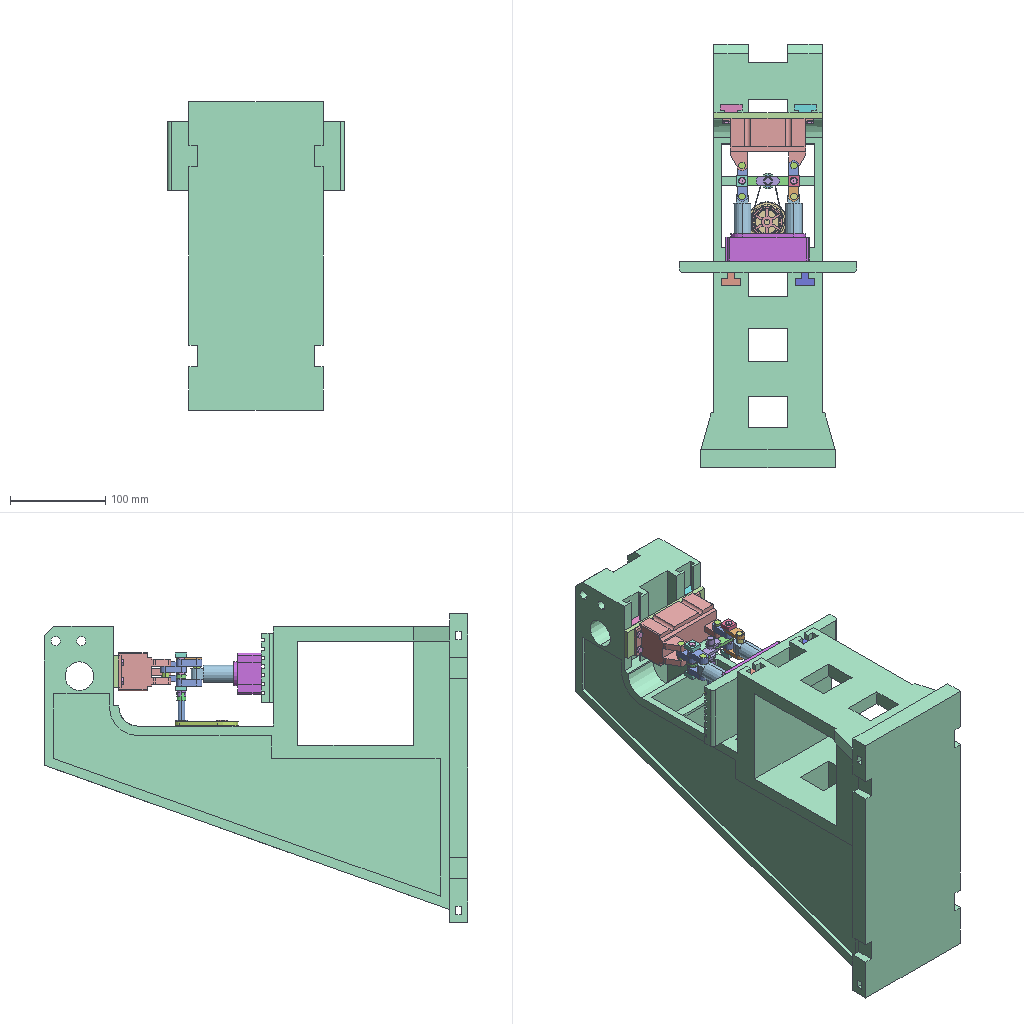Assembly | SolidWorks | 19 different items | 31 placed | box 186 x 445 x 325 mm
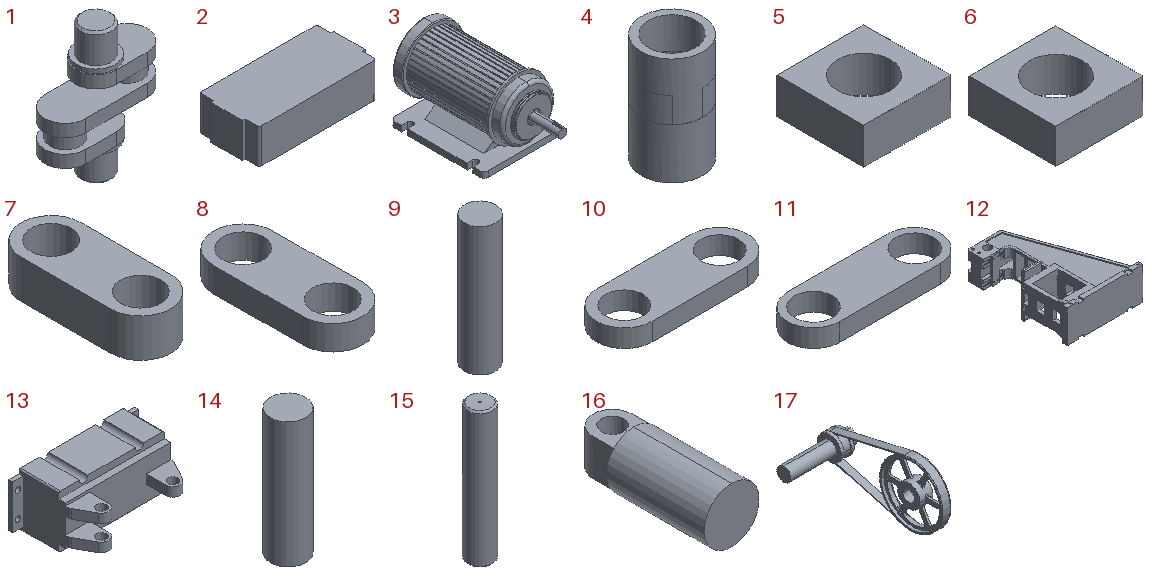Parts list (item | name | quantity | size | volume | features):
1 | - | x1 | 24.928 x 10.008 x 32 mm | 2653 mm3 | features ICE 9, Chamfer 1
2 | - | x1 | 88.335 x 43.022 x 29 mm | 100368 mm3 | features Extrusion 1, Fillet 1, ICE 1
3 | - | x1 | 55.501 x 97.908 x 48.521 mm | 103987 mm3 | features Cut 4, ICE 3, Extrusion 1, Fillet 1, Revolution 1
4 | - | x1 | 9.746 x 9.746 x 17 mm | 515.173 mm3 | features ICE 3, Extrusion 1
5 | - | x3 | 12 x 12 x 5 mm | 507.902 mm3 | features Extrusion 1
6 | - | x1 | 12 x 12 x 4.756 mm | 483.113 mm3 | features Extrusion 1
7 | - | x5 | 10.89 x 27.179 x 7 mm | 1300 mm3 | features Cut 2, Extrusion 1
8 | - | x2 | 11.013 x 27.178 x 4.5 mm | 835.586 mm3 | features Extrusion 1
9 | - | x1 | 7.349 x 7.349 x 30.108 mm | 1277 mm3 | features Extrusion 1
10 | - | x1 | 29.554 x 10.9 x 3.5 mm | 740.438 mm3 | features Extrusion 1
11 | - | x2 | 29.602 x 10.008 x 3.5 mm | 664.007 mm3 | features Cut 1, Extrusion 1
12 | - | x1 | 324.62 x 445 x 186.175 mm | 5513509 mm3 | features Cut 13, ICE 7, MoveFace 2, Chamfer 1, Extrusion 1, Fillet 1, MirrorPattern 1
13 | - | x1 | 95.251 x 55.228 x 40 mm | 112954 mm3 | features ICE 4, Cut 1, Extrusion 1, Fillet 1, MirrorPattern 1
14 | - | x3 | 7.349 x 7.349 x 26 mm | 1103 mm3 | features Extrusion 1
15 | - | x2 | 7.349 x 7.349 x 40 mm | 1691 mm3 | features Chamfer 1, Cut 1, Extrusion 1, MirrorPattern 1
16 | - | x2 | 18 x 45.316 x 18 mm | 9465 mm3 | features Cut 1, Extrusion 1, ICE 1
17 | - | x1 | 36 x 66.386 x 33.884 mm | 3751 mm3 | features ICE 6, Cut 2, Fillet 2, Extrusion 1
18 | hex nuts, style 1-grades ab gb | x1 | - | - | -
19 | hexagon head bolts-full thread gb | x1 | - | - | -
Mates (type | each side: item.copy, entity, surface, feature):
Concentric | 7.1 face cylinder Cut-Extrude1 | assembly face
Coincident | 13.1 face plane Boss-Extrude3 | assembly face
Concentric | 15.1 face cylinder Boss-Extrude1 | 7.2 face cylinder Cut-Extrude2
Coincident | 13.1 face plane Boss-Extrude3 | 7.2 face plane Boss-Extrude2
Concentric | 15.1 face cylinder Boss-Extrude1 | 7.3 face cylinder Cut-Extrude2
Coincident | 15.1 face cylinder Boss-Extrude1 | 5.1 edge
Coincident | 15.1 face plane Boss-Extrude1 | 5.1 face plane Boss-Extrude1
Parallel | 13.1 face plane Boss-Extrude1 | 5.1 face plane Boss-Extrude1
Concentric | 13.1 face cylinder Boss-Extrude4 | 14.1 face cylinder Boss-Extrude1
Coincident | 13.1 face plane Boss-Extrude3 | 14.1 face plane Boss-Extrude1
Concentric | 14.1 face cylinder Boss-Extrude1 | 7.4 face cylinder Cut-Extrude2
Concentric | 15.2 face cylinder Boss-Extrude1 | 7.4 face cylinder Cut-Extrude1
Coincident | 15.1 face plane Boss-Extrude1 | 15.2 face plane Boss-Extrude1
Concentric | 15.2 face cylinder Boss-Extrude1 | assembly face
Concentric | 15.2 face cylinder Boss-Extrude1 | 5.2 face cylinder Boss-Extrude1
Coincident | 15.2 face plane Boss-Extrude1 | assembly face
Coincident | 15.2 face plane Boss-Extrude1 | 5.2 face plane Boss-Extrude1
Concentric | 15.2 face cylinder Boss-Extrude1 | 7.5 face cylinder Cut-Extrude1
Coincident | 13.1 face plane Boss-Extrude4 | 7.4 face plane Boss-Extrude2
Coincident | 13.1 face plane Boss-Extrude4 | 7.5 face plane Boss-Extrude2
Concentric | 15.2 face cylinder Boss-Extrude1 | 8.1 face cylinder Boss-Extrude1
Coincident | 7.5 face plane Boss-Extrude2 | 8.1 face plane Boss-Extrude1
Concentric | 7.1 face cylinder Cut-Extrude2 | 14.2 face cylinder Boss-Extrude1
Coincident | 13.1 face plane Boss-Extrude3 | 7.1 face plane Boss-Extrude2
Coincident | 7.3 face plane Boss-Extrude2 | 5.1 face plane Boss-Extrude1
Concentric | 14.1 face cylinder Boss-Extrude1 | 7.5 face cylinder Cut-Extrude2
Concentric | 15.2 face cylinder Boss-Extrude1 | 8.2 face cylinder Boss-Extrude1
Concentric | 7.1 face cylinder Cut-Extrude1 | 15.1 face cylinder Boss-Extrude1
Concentric | 15.1 face cylinder Boss-Extrude1 | 11.1 face cylinder Cut-Extrude1
Concentric | 15.2 face cylinder Boss-Extrude1 | 11.2 face cylinder Cut-Extrude1
Concentric | 13.1 face cylinder Boss-Extrude3 | 14.2 face cylinder Boss-Extrude1
Concentric | 15.1 face cylinder Boss-Extrude1 | 5.3 face cylinder Boss-Extrude1
Coincident | 15.1 face plane Boss-Extrude1 | 5.3 face plane Boss-Extrude1
Coincident | 7.4 face plane Boss-Extrude2 | 11.2 face plane Boss-Extrude1
Concentric | 1.1 face cylinder Boss-Extrude8 | 11.1 face cylinder Cut-Extrude1
Concentric | 1.1 face cylinder Boss-Extrude9 | 11.2 face cylinder Cut-Extrude1
Coincident | 1.1 face plane Boss-Extrude11 | 11.2 face plane Boss-Extrude1
Concentric | 15.2 face cylinder Boss-Extrude1 | 6.1 face cylinder Boss-Extrude1
Coincident | 8.2 face plane Boss-Extrude1 | 6.1 face plane Boss-Extrude1
Coincident | 5.2 face plane Boss-Extrude1 | 8.1 face plane Boss-Extrude1
Coincident | 1.1 face plane Boss-Extrude7 | 11.1 face plane Boss-Extrude1
Concentric | 7.3 face cylinder Cut-Extrude1 | 16.1 face cylinder Cut-Extrude1
Coincident | 16.2 face plane Boss-Extrude1 | 16.1 face plane Boss-Extrude1
Concentric | 7.3 face cylinder Cut-Extrude1 | 14.3 face cylinder Boss-Extrude1
Coincident | 7.2 face plane Boss-Extrude2 | 14.3 face plane Boss-Extrude1
Concentric | 16.1 face cylinder Boss-Extrude2 | 2.1 face cylinder Boss-Extrude1
Concentric | 16.2 face cylinder Boss-Extrude2 | 2.1 face cylinder Boss-Extrude1
Coincident | 16.1 face plane Boss-Extrude2 | 2.1 face plane Boss-Extrude1
Concentric | 7.2 face cylinder Cut-Extrude1 | 14.3 face cylinder Boss-Extrude1
Concentric | 8.2 face cylinder Boss-Extrude1 | 9.1 face cylinder Boss-Extrude1
Concentric | 8.1 face cylinder Boss-Extrude1 | 9.1 face cylinder Boss-Extrude1
Parallel | 16.2 face cylinder Cut-Extrude1 | 9.1 face cylinder Boss-Extrude1
Concentric | 16.2 face cylinder Cut-Extrude1 | 9.1 face cylinder Boss-Extrude1
Coincident | 7.4 face plane Boss-Extrude2 | 8.2 face plane Boss-Extrude1
Coincident | 7.3 face plane Boss-Extrude2 | 16.1 face plane Boss-Extrude1
Coincident | 16.2 face plane Boss-Extrude2 | 2.1 face plane Boss-Extrude1
Parallel | 2.1 face plane Boss-Extrude2 | assembly plane